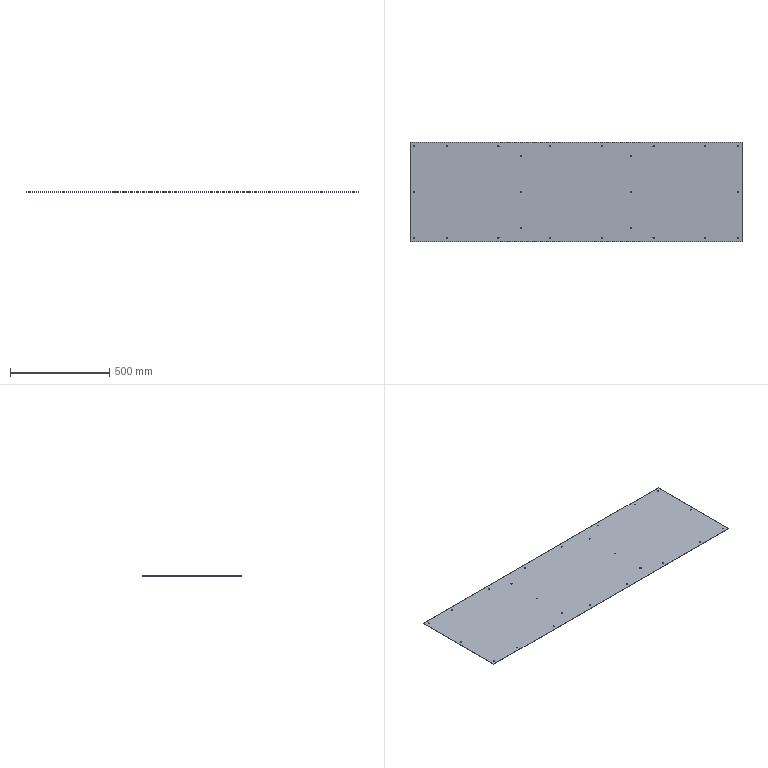Part | STEP file | TS-S92 | 1 solid | 54 faces | box 1670 x 502 x 1.2 mm | volume 1005348 mm3 | cylinder 48 | plane 6 | commonest cylinder face diameters 5.4 x48